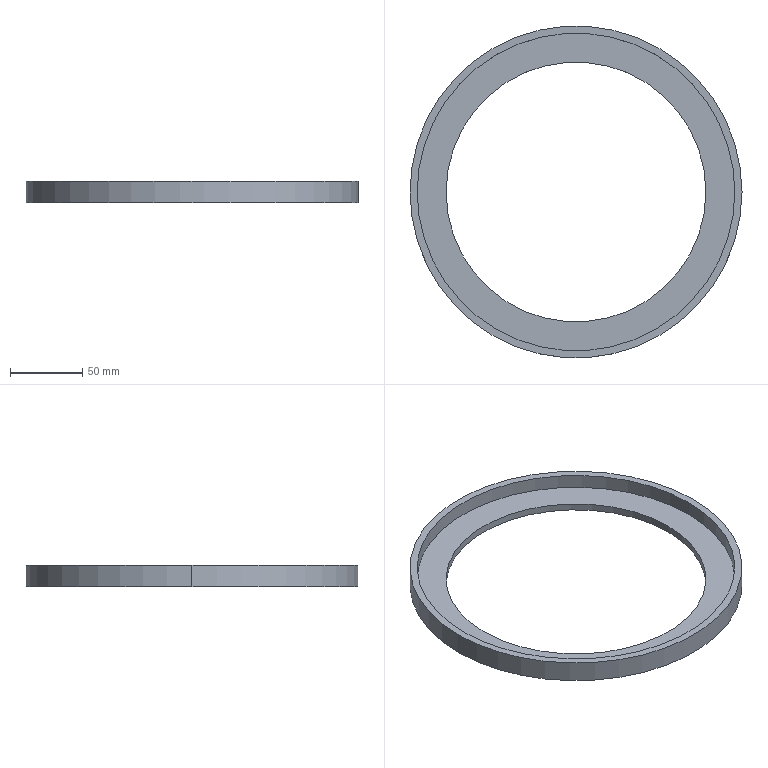Part | SolidWorks | features ICE 5, Cut 1, Extrusion 1 | 1 solid | 9 faces | box 230 x 230 x 15 mm | volume 115846 mm3 | cylinder 6 | plane 3 | commonest cylinder face diameters 180 x2 220 x2 230 x2
STEP:
#1=CARTESIAN_POINT('',(-90.,0.,0.));
#2=VERTEX_POINT('',#1);
#3=CARTESIAN_POINT('',(90.,0.,0.));
#4=VERTEX_POINT('',#3);
#5=CARTESIAN_POINT('',(0.,0.,0.));
#6=DIRECTION('',(0.,0.,1.));
#7=DIRECTION('',(1.,0.,0.));
#8=AXIS2_PLACEMENT_3D('',#5,#6,#7);
#9=CIRCLE('',#8,90.);
#10=EDGE_CURVE('',#2,#4,#9,.T.);
#11=ORIENTED_EDGE('',*,*,#10,.F.);
#12=CARTESIAN_POINT('',(-90.,0.,5.));
#13=VERTEX_POINT('',#12);
#14=CARTESIAN_POINT('',(-90.,0.,-43.));
#15=DIRECTION('',(0.,0.,1.));
#16=VECTOR('',#15,1000.);
#17=LINE('',#14,#16);
#18=EDGE_CURVE('',#2,#13,#17,.T.);
#19=ORIENTED_EDGE('',*,*,#18,.T.);
#20=CARTESIAN_POINT('',(90.,0.,5.));
#21=VERTEX_POINT('',#20);
#22=CARTESIAN_POINT('',(0.,0.,5.));
#23=DIRECTION('',(0.,0.,-1.));
#24=DIRECTION('',(1.,0.,0.));
#25=AXIS2_PLACEMENT_3D('',#22,#23,#24);
#26=CIRCLE('',#25,90.);
#27=EDGE_CURVE('',#21,#13,#26,.T.);
#28=ORIENTED_EDGE('',*,*,#27,.F.);
#29=CARTESIAN_POINT('',(90.,0.,-43.));
#30=DIRECTION('',(0.,0.,1.));
#31=VECTOR('',#30,1000.);
#32=LINE('',#29,#31);
#33=EDGE_CURVE('',#4,#21,#32,.T.);
#34=ORIENTED_EDGE('',*,*,#33,.F.);
#35=EDGE_LOOP('',(#11,#19,#28,#34));
#36=FACE_OUTER_BOUND('',#35,.T.);
#37=CARTESIAN_POINT('',(0.,0.,-43.));
#38=DIRECTION('',(0.,0.,1.));
#39=DIRECTION('',(1.,0.,0.));
#40=AXIS2_PLACEMENT_3D('',#37,#38,#39);
#41=CYLINDRICAL_SURFACE('',#40,90.);
#42=ADVANCED_FACE('',(#36),#41,.F.);
#43=CARTESIAN_POINT('',(115.,0.,0.));
#44=VERTEX_POINT('',#43);
#45=CARTESIAN_POINT('',(-115.,0.,0.));
#46=VERTEX_POINT('',#45);
#47=CARTESIAN_POINT('',(0.,0.,0.));
#48=DIRECTION('',(0.,0.,1.));
#49=DIRECTION('',(1.,0.,0.));
#50=AXIS2_PLACEMENT_3D('',#47,#48,#49);
#51=CIRCLE('',#50,115.);
#52=EDGE_CURVE('',#44,#46,#51,.T.);
#53=ORIENTED_EDGE('',*,*,#52,.T.);
#54=CARTESIAN_POINT('',(-115.,0.,15.));
#55=VERTEX_POINT('',#54);
#56=CARTESIAN_POINT('',(-115.,0.,0.));
#57=DIRECTION('',(0.,0.,1.));
#58=VECTOR('',#57,1000.);
#59=LINE('',#56,#58);
#60=EDGE_CURVE('',#46,#55,#59,.T.);
#61=ORIENTED_EDGE('',*,*,#60,.T.);
#62=CARTESIAN_POINT('',(115.,0.,15.));
#63=VERTEX_POINT('',#62);
#64=CARTESIAN_POINT('',(0.,0.,15.));
#65=DIRECTION('',(0.,0.,-1.));
#66=DIRECTION('',(1.,0.,0.));
#67=AXIS2_PLACEMENT_3D('',#64,#65,#66);
#68=CIRCLE('',#67,115.);
#69=EDGE_CURVE('',#55,#63,#68,.T.);
#70=ORIENTED_EDGE('',*,*,#69,.T.);
#71=CARTESIAN_POINT('',(115.,0.,0.));
#72=DIRECTION('',(0.,0.,1.));
#73=VECTOR('',#72,1000.);
#74=LINE('',#71,#73);
#75=EDGE_CURVE('',#44,#63,#74,.T.);
#76=ORIENTED_EDGE('',*,*,#75,.F.);
#77=EDGE_LOOP('',(#53,#61,#70,#76));
#78=FACE_OUTER_BOUND('',#77,.T.);
#79=CARTESIAN_POINT('',(0.,0.,0.));
#80=DIRECTION('',(0.,0.,1.));
#81=DIRECTION('',(1.,0.,0.));
#82=AXIS2_PLACEMENT_3D('',#79,#80,#81);
#83=CYLINDRICAL_SURFACE('',#82,115.);
#84=ADVANCED_FACE('',(#78),#83,.T.);
#85=CARTESIAN_POINT('',(-110.,0.,5.));
#86=VERTEX_POINT('',#85);
#87=CARTESIAN_POINT('',(110.,0.,5.));
#88=VERTEX_POINT('',#87);
#89=CARTESIAN_POINT('',(0.,0.,5.));
#90=DIRECTION('',(0.,0.,1.));
#91=DIRECTION('',(-1.,0.,0.));
#92=AXIS2_PLACEMENT_3D('',#89,#90,#91);
#93=CIRCLE('',#92,110.);
#94=EDGE_CURVE('',#86,#88,#93,.T.);
#95=ORIENTED_EDGE('',*,*,#94,.F.);
#96=CARTESIAN_POINT('',(-110.,0.,15.));
#97=VERTEX_POINT('',#96);
#98=CARTESIAN_POINT('',(-110.,0.,0.));
#99=DIRECTION('',(0.,0.,1.));
#100=VECTOR('',#99,1000.);
#101=LINE('',#98,#100);
#102=EDGE_CURVE('',#86,#97,#101,.T.);
#103=ORIENTED_EDGE('',*,*,#102,.T.);
#104=CARTESIAN_POINT('',(110.,0.,15.));
#105=VERTEX_POINT('',#104);
#106=CARTESIAN_POINT('',(0.,0.,15.));
#107=DIRECTION('',(0.,0.,-1.));
#108=DIRECTION('',(1.,0.,0.));
#109=AXIS2_PLACEMENT_3D('',#106,#107,#108);
#110=CIRCLE('',#109,110.);
#111=EDGE_CURVE('',#105,#97,#110,.T.);
#112=ORIENTED_EDGE('',*,*,#111,.F.);
#113=CARTESIAN_POINT('',(110.,0.,0.));
#114=DIRECTION('',(0.,0.,1.));
#115=VECTOR('',#114,1000.);
#116=LINE('',#113,#115);
#117=EDGE_CURVE('',#88,#105,#116,.T.);
#118=ORIENTED_EDGE('',*,*,#117,.F.);
#119=EDGE_LOOP('',(#95,#103,#112,#118));
#120=FACE_OUTER_BOUND('',#119,.T.);
#121=CARTESIAN_POINT('',(0.,0.,0.));
#122=DIRECTION('',(0.,0.,1.));
#123=DIRECTION('',(1.,0.,0.));
#124=AXIS2_PLACEMENT_3D('',#121,#122,#123);
#125=CYLINDRICAL_SURFACE('',#124,110.);
#126=ADVANCED_FACE('',(#120),#125,.F.);
#127=ORIENTED_EDGE('',*,*,#102,.F.);
#128=CARTESIAN_POINT('',(0.,0.,5.));
#129=DIRECTION('',(0.,0.,1.));
#130=DIRECTION('',(-1.,0.,0.));
#131=AXIS2_PLACEMENT_3D('',#128,#129,#130);
#132=CIRCLE('',#131,110.);
#133=EDGE_CURVE('',#88,#86,#132,.T.);
#134=ORIENTED_EDGE('',*,*,#133,.F.);
#135=ORIENTED_EDGE('',*,*,#117,.T.);
#136=CARTESIAN_POINT('',(0.,0.,15.));
#137=DIRECTION('',(0.,0.,-1.));
#138=DIRECTION('',(1.,0.,0.));
#139=AXIS2_PLACEMENT_3D('',#136,#137,#138);
#140=CIRCLE('',#139,110.);
#141=EDGE_CURVE('',#97,#105,#140,.T.);
#142=ORIENTED_EDGE('',*,*,#141,.F.);
#143=EDGE_LOOP('',(#127,#134,#135,#142));
#144=FACE_OUTER_BOUND('',#143,.T.);
#145=CARTESIAN_POINT('',(0.,0.,0.));
#146=DIRECTION('',(0.,0.,1.));
#147=DIRECTION('',(1.,0.,0.));
#148=AXIS2_PLACEMENT_3D('',#145,#146,#147);
#149=CYLINDRICAL_SURFACE('',#148,110.);
#150=ADVANCED_FACE('',(#144),#149,.F.);
#151=ORIENTED_EDGE('',*,*,#60,.F.);
#152=CARTESIAN_POINT('',(0.,0.,0.));
#153=DIRECTION('',(0.,0.,1.));
#154=DIRECTION('',(1.,0.,0.));
#155=AXIS2_PLACEMENT_3D('',#152,#153,#154);
#156=CIRCLE('',#155,115.);
#157=EDGE_CURVE('',#46,#44,#156,.T.);
#158=ORIENTED_EDGE('',*,*,#157,.T.);
#159=ORIENTED_EDGE('',*,*,#75,.T.);
#160=CARTESIAN_POINT('',(0.,0.,15.));
#161=DIRECTION('',(0.,0.,-1.));
#162=DIRECTION('',(1.,0.,0.));
#163=AXIS2_PLACEMENT_3D('',#160,#161,#162);
#164=CIRCLE('',#163,115.);
#165=EDGE_CURVE('',#63,#55,#164,.T.);
#166=ORIENTED_EDGE('',*,*,#165,.T.);
#167=EDGE_LOOP('',(#151,#158,#159,#166));
#168=FACE_OUTER_BOUND('',#167,.T.);
#169=CARTESIAN_POINT('',(0.,0.,0.));
#170=DIRECTION('',(0.,0.,1.));
#171=DIRECTION('',(1.,0.,0.));
#172=AXIS2_PLACEMENT_3D('',#169,#170,#171);
#173=CYLINDRICAL_SURFACE('',#172,115.);
#174=ADVANCED_FACE('',(#168),#173,.T.);
#175=ORIENTED_EDGE('',*,*,#52,.F.);
#176=ORIENTED_EDGE('',*,*,#157,.F.);
#177=EDGE_LOOP('',(#175,#176));
#178=FACE_OUTER_BOUND('',#177,.T.);
#179=CARTESIAN_POINT('',(0.,0.,0.));
#180=DIRECTION('',(0.,0.,1.));
#181=DIRECTION('',(1.,0.,0.));
#182=AXIS2_PLACEMENT_3D('',#179,#180,#181);
#183=CIRCLE('',#182,90.);
#184=EDGE_CURVE('',#4,#2,#183,.T.);
#185=ORIENTED_EDGE('',*,*,#184,.T.);
#186=ORIENTED_EDGE('',*,*,#10,.T.);
#187=EDGE_LOOP('',(#185,#186));
#188=FACE_BOUND('',#187,.T.);
#189=CARTESIAN_POINT('',(0.,0.,0.));
#190=DIRECTION('',(0.,0.,1.));
#191=DIRECTION('',(1.,0.,0.));
#192=AXIS2_PLACEMENT_3D('',#189,#190,#191);
#193=PLANE('',#192);
#194=ADVANCED_FACE('',(#178,#188),#193,.F.);
#195=ORIENTED_EDGE('',*,*,#133,.T.);
#196=ORIENTED_EDGE('',*,*,#94,.T.);
#197=EDGE_LOOP('',(#195,#196));
#198=FACE_OUTER_BOUND('',#197,.T.);
#199=ORIENTED_EDGE('',*,*,#27,.T.);
#200=CARTESIAN_POINT('',(0.,0.,5.));
#201=DIRECTION('',(0.,0.,-1.));
#202=DIRECTION('',(1.,0.,0.));
#203=AXIS2_PLACEMENT_3D('',#200,#201,#202);
#204=CIRCLE('',#203,90.);
#205=EDGE_CURVE('',#13,#21,#204,.T.);
#206=ORIENTED_EDGE('',*,*,#205,.T.);
#207=EDGE_LOOP('',(#199,#206));
#208=FACE_BOUND('',#207,.T.);
#209=CARTESIAN_POINT('',(0.,0.,5.));
#210=DIRECTION('',(0.,0.,-1.));
#211=DIRECTION('',(-1.,0.,0.));
#212=AXIS2_PLACEMENT_3D('',#209,#210,#211);
#213=PLANE('',#212);
#214=ADVANCED_FACE('',(#198,#208),#213,.F.);
#215=ORIENTED_EDGE('',*,*,#18,.F.);
#216=ORIENTED_EDGE('',*,*,#184,.F.);
#217=ORIENTED_EDGE('',*,*,#33,.T.);
#218=ORIENTED_EDGE('',*,*,#205,.F.);
#219=EDGE_LOOP('',(#215,#216,#217,#218));
#220=FACE_OUTER_BOUND('',#219,.T.);
#221=CARTESIAN_POINT('',(0.,0.,-43.));
#222=DIRECTION('',(0.,0.,1.));
#223=DIRECTION('',(1.,0.,0.));
#224=AXIS2_PLACEMENT_3D('',#221,#222,#223);
#225=CYLINDRICAL_SURFACE('',#224,90.);
#226=ADVANCED_FACE('',(#220),#225,.F.);
#227=ORIENTED_EDGE('',*,*,#165,.F.);
#228=ORIENTED_EDGE('',*,*,#69,.F.);
#229=EDGE_LOOP('',(#227,#228));
#230=FACE_OUTER_BOUND('',#229,.T.);
#231=ORIENTED_EDGE('',*,*,#111,.T.);
#232=ORIENTED_EDGE('',*,*,#141,.T.);
#233=EDGE_LOOP('',(#231,#232));
#234=FACE_BOUND('',#233,.T.);
#235=CARTESIAN_POINT('',(0.,0.,15.));
#236=DIRECTION('',(0.,0.,1.));
#237=DIRECTION('',(1.,0.,0.));
#238=AXIS2_PLACEMENT_3D('',#235,#236,#237);
#239=PLANE('',#238);
#240=ADVANCED_FACE('',(#230,#234),#239,.T.);
#241=CLOSED_SHELL('',(#42,#84,#126,#150,#174,#194,#214,#226,#240));
#242=MANIFOLD_SOLID_BREP('',#241);
#243=CARTESIAN_POINT('',(0.,0.,0.));
#244=DIRECTION('',(0.,0.,1.));
#245=DIRECTION('',(1.,0.,0.));
#246=AXIS2_PLACEMENT_3D('',#243,#244,#245);
#247=(LENGTH_UNIT()NAMED_UNIT(*)SI_UNIT(.MILLI.,.METRE.));
#248=UNCERTAINTY_MEASURE_WITH_UNIT(LENGTH_MEASURE(0.00001),#247,'','');
#249=(NAMED_UNIT(*)PLANE_ANGLE_UNIT()SI_UNIT($,.RADIAN.));
#250=(NAMED_UNIT(*)SI_UNIT($,.STERADIAN.)SOLID_ANGLE_UNIT());
#251=(GEOMETRIC_REPRESENTATION_CONTEXT(3)GLOBAL_UNCERTAINTY_ASSIGNED_CONTEXT((#248))GLOBAL_UNIT_ASSIGNED_CONTEXT((#247,#249,#250))REPRESENTATION_CONTEXT('',''));
#252=ADVANCED_BREP_SHAPE_REPRESENTATION('',(#242,#246),#251);